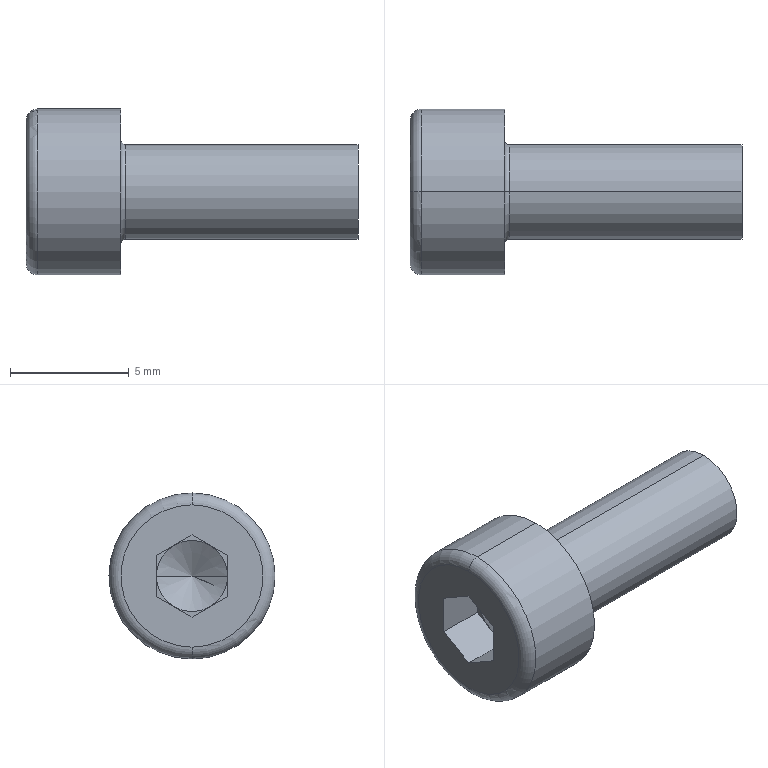Part | NX | features BREP 1 | 1 solid | 25 faces | box 14 x 7 x 7 mm | volume 260.941 mm3 | plane 15 | torus 4 | cylinder 4 | cone 2 | commonest cylinder face diameters 4 x2 7 x2
STEP:
#1=CARTESIAN_POINT('',(0.5,0.,-3.5));
#2=VERTEX_POINT('',#1);
#3=CARTESIAN_POINT('',(0.5,0.,3.5));
#4=VERTEX_POINT('',#3);
#5=CARTESIAN_POINT('',(0.5,0.,0.));
#6=DIRECTION('',(1.,0.,0.));
#7=DIRECTION('',(0.,0.,1.));
#8=AXIS2_PLACEMENT_3D('',#5,#6,#7);
#9=CIRCLE('',#8,3.5);
#10=EDGE_CURVE('',#2,#4,#9,.T.);
#11=ORIENTED_EDGE('',*,*,#10,.F.);
#12=CARTESIAN_POINT('',(0.,0.,-3.));
#13=VERTEX_POINT('',#12);
#14=CARTESIAN_POINT('',(0.5,0.,-3.));
#15=DIRECTION('',(0.,1.,0.));
#16=DIRECTION('',(0.,0.,1.));
#17=AXIS2_PLACEMENT_3D('',#14,#15,#16);
#18=CIRCLE('',#17,0.5);
#19=EDGE_CURVE('',#2,#13,#18,.T.);
#20=ORIENTED_EDGE('',*,*,#19,.T.);
#21=CARTESIAN_POINT('',(0.,0.,3.));
#22=VERTEX_POINT('',#21);
#23=CARTESIAN_POINT('',(0.,0.,0.));
#24=DIRECTION('',(-1.,0.,0.));
#25=DIRECTION('',(0.,0.,1.));
#26=AXIS2_PLACEMENT_3D('',#23,#24,#25);
#27=CIRCLE('',#26,3.);
#28=EDGE_CURVE('',#22,#13,#27,.T.);
#29=ORIENTED_EDGE('',*,*,#28,.F.);
#30=CARTESIAN_POINT('',(0.5,0.,3.));
#31=DIRECTION('',(0.,-1.,0.));
#32=DIRECTION('',(0.,0.,-1.));
#33=AXIS2_PLACEMENT_3D('',#30,#31,#32);
#34=CIRCLE('',#33,0.5);
#35=EDGE_CURVE('',#4,#22,#34,.T.);
#36=ORIENTED_EDGE('',*,*,#35,.F.);
#37=EDGE_LOOP('',(#11,#20,#29,#36));
#38=FACE_BOUND('',#37,.T.);
#39=CARTESIAN_POINT('',(0.5,0.,0.));
#40=DIRECTION('',(-1.,0.,0.));
#41=DIRECTION('',(0.,0.,-1.));
#42=AXIS2_PLACEMENT_3D('',#39,#40,#41);
#43=TOROIDAL_SURFACE('',#42,3.,0.5);
#44=ADVANCED_FACE('',(#38),#43,.T.);
#45=CARTESIAN_POINT('',(4.2,0.,2.));
#46=VERTEX_POINT('',#45);
#47=CARTESIAN_POINT('',(4.2,0.,-2.));
#48=VERTEX_POINT('',#47);
#49=CARTESIAN_POINT('',(4.2,0.,0.));
#50=DIRECTION('',(1.,0.,0.));
#51=DIRECTION('',(0.,0.,-1.));
#52=AXIS2_PLACEMENT_3D('',#49,#50,#51);
#53=CIRCLE('',#52,2.);
#54=EDGE_CURVE('',#46,#48,#53,.T.);
#55=ORIENTED_EDGE('',*,*,#54,.F.);
#56=CARTESIAN_POINT('',(4.,0.,2.2));
#57=VERTEX_POINT('',#56);
#58=CARTESIAN_POINT('',(4.2,0.,2.2));
#59=DIRECTION('',(0.,1.,0.));
#60=DIRECTION('',(0.,0.,1.));
#61=AXIS2_PLACEMENT_3D('',#58,#59,#60);
#62=CIRCLE('',#61,0.2);
#63=EDGE_CURVE('',#57,#46,#62,.F.);
#64=ORIENTED_EDGE('',*,*,#63,.F.);
#65=CARTESIAN_POINT('',(4.,0.,-2.2));
#66=VERTEX_POINT('',#65);
#67=CARTESIAN_POINT('',(4.,0.,0.));
#68=DIRECTION('',(-1.,0.,0.));
#69=DIRECTION('',(0.,0.,-1.));
#70=AXIS2_PLACEMENT_3D('',#67,#68,#69);
#71=CIRCLE('',#70,2.2);
#72=EDGE_CURVE('',#66,#57,#71,.T.);
#73=ORIENTED_EDGE('',*,*,#72,.F.);
#74=CARTESIAN_POINT('',(4.2,0.,-2.2));
#75=DIRECTION('',(0.,-1.,0.));
#76=DIRECTION('',(0.,0.,-1.));
#77=AXIS2_PLACEMENT_3D('',#74,#75,#76);
#78=CIRCLE('',#77,0.2);
#79=EDGE_CURVE('',#66,#48,#78,.F.);
#80=ORIENTED_EDGE('',*,*,#79,.T.);
#81=EDGE_LOOP('',(#55,#64,#73,#80));
#82=FACE_BOUND('',#81,.T.);
#83=CARTESIAN_POINT('',(4.2,0.,0.));
#84=DIRECTION('',(1.,0.,0.));
#85=DIRECTION('',(0.,0.,1.));
#86=AXIS2_PLACEMENT_3D('',#83,#84,#85);
#87=TOROIDAL_SURFACE('',#86,2.2,0.2);
#88=ADVANCED_FACE('',(#82),#87,.F.);
#89=CARTESIAN_POINT('',(2.,-1.5,0.));
#90=VERTEX_POINT('',#89);
#91=CARTESIAN_POINT('',(2.866,0.,0.));
#92=VERTEX_POINT('',#91);
#93=CARTESIAN_POINT('',(2.866,0.,0.));
#94=DIRECTION('',(-0.5,-0.866,0.));
#95=VECTOR('',#94,1000.);
#96=LINE('',#93,#95);
#97=EDGE_CURVE('',#90,#92,#96,.F.);
#98=ORIENTED_EDGE('',*,*,#97,.T.);
#99=CARTESIAN_POINT('',(2.,1.5,0.));
#100=VERTEX_POINT('',#99);
#101=CARTESIAN_POINT('',(2.866,0.,0.));
#102=DIRECTION('',(-0.5,0.866,0.));
#103=VECTOR('',#102,1000.);
#104=LINE('',#101,#103);
#105=EDGE_CURVE('',#100,#92,#104,.F.);
#106=ORIENTED_EDGE('',*,*,#105,.F.);
#107=CARTESIAN_POINT('',(2.,0.75,-1.299));
#108=VERTEX_POINT('',#107);
#109=CARTESIAN_POINT('',(2.,0.,0.));
#110=DIRECTION('',(1.,0.,0.));
#111=DIRECTION('',(0.,1.,0.));
#112=AXIS2_PLACEMENT_3D('',#109,#110,#111);
#113=CIRCLE('',#112,1.5);
#114=EDGE_CURVE('',#108,#100,#113,.T.);
#115=ORIENTED_EDGE('',*,*,#114,.F.);
#116=CARTESIAN_POINT('',(2.,-0.75,-1.299));
#117=VERTEX_POINT('',#116);
#118=CARTESIAN_POINT('',(2.,0.,0.));
#119=DIRECTION('',(1.,0.,0.));
#120=DIRECTION('',(0.,1.,0.));
#121=AXIS2_PLACEMENT_3D('',#118,#119,#120);
#122=CIRCLE('',#121,1.5);
#123=EDGE_CURVE('',#117,#108,#122,.T.);
#124=ORIENTED_EDGE('',*,*,#123,.F.);
#125=CARTESIAN_POINT('',(2.,0.,0.));
#126=DIRECTION('',(1.,0.,0.));
#127=DIRECTION('',(0.,1.,0.));
#128=AXIS2_PLACEMENT_3D('',#125,#126,#127);
#129=CIRCLE('',#128,1.5);
#130=EDGE_CURVE('',#90,#117,#129,.T.);
#131=ORIENTED_EDGE('',*,*,#130,.F.);
#132=EDGE_LOOP('',(#98,#106,#115,#124,#131));
#133=FACE_BOUND('',#132,.T.);
#134=CARTESIAN_POINT('',(-997.134,0.,0.));
#135=DIRECTION('',(-1.,0.,0.));
#136=DIRECTION('',(0.,1.,0.));
#137=AXIS2_PLACEMENT_3D('',#134,#135,#136);
#138=CONICAL_SURFACE('',#137,1732.051,1.047);
#139=ADVANCED_FACE('',(#133),#138,.F.);
#140=CARTESIAN_POINT('',(14.,0.,-2.));
#141=VERTEX_POINT('',#140);
#142=CARTESIAN_POINT('',(14.,0.,2.));
#143=VERTEX_POINT('',#142);
#144=CARTESIAN_POINT('',(14.,0.,0.));
#145=DIRECTION('',(1.,0.,0.));
#146=DIRECTION('',(0.,0.,-1.));
#147=AXIS2_PLACEMENT_3D('',#144,#145,#146);
#148=CIRCLE('',#147,2.);
#149=EDGE_CURVE('',#141,#143,#148,.T.);
#150=ORIENTED_EDGE('',*,*,#149,.F.);
#151=CARTESIAN_POINT('',(10.,0.,-2.));
#152=DIRECTION('',(-1.,0.,0.));
#153=VECTOR('',#152,1000.);
#154=LINE('',#151,#153);
#155=EDGE_CURVE('',#141,#48,#154,.T.);
#156=ORIENTED_EDGE('',*,*,#155,.T.);
#157=CARTESIAN_POINT('',(4.2,0.,0.));
#158=DIRECTION('',(1.,0.,0.));
#159=DIRECTION('',(0.,0.,-1.));
#160=AXIS2_PLACEMENT_3D('',#157,#158,#159);
#161=CIRCLE('',#160,2.);
#162=EDGE_CURVE('',#48,#46,#161,.T.);
#163=ORIENTED_EDGE('',*,*,#162,.T.);
#164=CARTESIAN_POINT('',(10.,0.,2.));
#165=DIRECTION('',(-1.,0.,0.));
#166=VECTOR('',#165,1000.);
#167=LINE('',#164,#166);
#168=EDGE_CURVE('',#143,#46,#167,.T.);
#169=ORIENTED_EDGE('',*,*,#168,.F.);
#170=EDGE_LOOP('',(#150,#156,#163,#169));
#171=FACE_BOUND('',#170,.T.);
#172=CARTESIAN_POINT('',(10.,0.,0.));
#173=DIRECTION('',(-1.,0.,0.));
#174=DIRECTION('',(0.,0.,-1.));
#175=AXIS2_PLACEMENT_3D('',#172,#173,#174);
#176=CYLINDRICAL_SURFACE('',#175,2.);
#177=ADVANCED_FACE('',(#171),#176,.T.);
#178=CARTESIAN_POINT('',(4.,0.,3.5));
#179=VERTEX_POINT('',#178);
#180=CARTESIAN_POINT('',(4.,0.,-3.5));
#181=VERTEX_POINT('',#180);
#182=CARTESIAN_POINT('',(4.,0.,0.));
#183=DIRECTION('',(-1.,0.,0.));
#184=DIRECTION('',(0.,0.,1.));
#185=AXIS2_PLACEMENT_3D('',#182,#183,#184);
#186=CIRCLE('',#185,3.5);
#187=EDGE_CURVE('',#179,#181,#186,.T.);
#188=ORIENTED_EDGE('',*,*,#187,.T.);
#189=CARTESIAN_POINT('',(4.,0.,-3.5));
#190=DIRECTION('',(-1.,0.,0.));
#191=VECTOR('',#190,1000.);
#192=LINE('',#189,#191);
#193=EDGE_CURVE('',#181,#2,#192,.T.);
#194=ORIENTED_EDGE('',*,*,#193,.T.);
#195=ORIENTED_EDGE('',*,*,#10,.T.);
#196=CARTESIAN_POINT('',(4.,0.,3.5));
#197=DIRECTION('',(-1.,0.,0.));
#198=VECTOR('',#197,1000.);
#199=LINE('',#196,#198);
#200=EDGE_CURVE('',#179,#4,#199,.T.);
#201=ORIENTED_EDGE('',*,*,#200,.F.);
#202=EDGE_LOOP('',(#188,#194,#195,#201));
#203=FACE_BOUND('',#202,.T.);
#204=CARTESIAN_POINT('',(4.,0.,0.));
#205=DIRECTION('',(-1.,0.,0.));
#206=DIRECTION('',(0.,0.,-1.));
#207=AXIS2_PLACEMENT_3D('',#204,#205,#206);
#208=CYLINDRICAL_SURFACE('',#207,3.5);
#209=ADVANCED_FACE('',(#203),#208,.T.);
#210=CARTESIAN_POINT('',(2.,1.5,0.866));
#211=VERTEX_POINT('',#210);
#212=CARTESIAN_POINT('',(2.,1.5,0.866));
#213=DIRECTION('',(0.,0.,-1.));
#214=VECTOR('',#213,1000.);
#215=LINE('',#212,#214);
#216=EDGE_CURVE('',#211,#100,#215,.T.);
#217=ORIENTED_EDGE('',*,*,#216,.T.);
#218=CARTESIAN_POINT('',(2.,0.75,1.299));
#219=VERTEX_POINT('',#218);
#220=CARTESIAN_POINT('',(2.,0.,0.));
#221=DIRECTION('',(1.,0.,0.));
#222=DIRECTION('',(0.,1.,0.));
#223=AXIS2_PLACEMENT_3D('',#220,#221,#222);
#224=CIRCLE('',#223,1.5);
#225=EDGE_CURVE('',#100,#219,#224,.T.);
#226=ORIENTED_EDGE('',*,*,#225,.T.);
#227=CARTESIAN_POINT('',(2.,0.,1.732));
#228=DIRECTION('',(0.,0.866,-0.5));
#229=VECTOR('',#228,1000.);
#230=LINE('',#227,#229);
#231=EDGE_CURVE('',#219,#211,#230,.T.);
#232=ORIENTED_EDGE('',*,*,#231,.T.);
#233=EDGE_LOOP('',(#217,#226,#232));
#234=FACE_BOUND('',#233,.T.);
#235=CARTESIAN_POINT('',(2.,0.,0.));
#236=DIRECTION('',(-1.,0.,0.));
#237=DIRECTION('',(0.,0.,-1.));
#238=AXIS2_PLACEMENT_3D('',#235,#236,#237);
#239=PLANE('',#238);
#240=ADVANCED_FACE('',(#234),#239,.T.);
#241=CARTESIAN_POINT('',(2.,0.,1.732));
#242=VERTEX_POINT('',#241);
#243=CARTESIAN_POINT('',(2.,0.,1.732));
#244=DIRECTION('',(0.,0.866,-0.5));
#245=VECTOR('',#244,1000.);
#246=LINE('',#243,#245);
#247=EDGE_CURVE('',#242,#219,#246,.T.);
#248=ORIENTED_EDGE('',*,*,#247,.T.);
#249=CARTESIAN_POINT('',(2.,-0.75,1.299));
#250=VERTEX_POINT('',#249);
#251=CARTESIAN_POINT('',(2.,0.,0.));
#252=DIRECTION('',(1.,0.,0.));
#253=DIRECTION('',(0.,1.,0.));
#254=AXIS2_PLACEMENT_3D('',#251,#252,#253);
#255=CIRCLE('',#254,1.5);
#256=EDGE_CURVE('',#219,#250,#255,.T.);
#257=ORIENTED_EDGE('',*,*,#256,.T.);
#258=CARTESIAN_POINT('',(2.,-1.5,0.866));
#259=DIRECTION('',(0.,0.866,0.5));
#260=VECTOR('',#259,1000.);
#261=LINE('',#258,#260);
#262=EDGE_CURVE('',#250,#242,#261,.T.);
#263=ORIENTED_EDGE('',*,*,#262,.T.);
#264=EDGE_LOOP('',(#248,#257,#263));
#265=FACE_BOUND('',#264,.T.);
#266=CARTESIAN_POINT('',(2.,0.,0.));
#267=DIRECTION('',(-1.,0.,0.));
#268=DIRECTION('',(0.,0.,-1.));
#269=AXIS2_PLACEMENT_3D('',#266,#267,#268);
#270=PLANE('',#269);
#271=ADVANCED_FACE('',(#265),#270,.T.);
#272=CARTESIAN_POINT('',(2.,-1.5,0.866));
#273=VERTEX_POINT('',#272);
#274=CARTESIAN_POINT('',(2.,-1.5,0.866));
#275=DIRECTION('',(0.,0.866,0.5));
#276=VECTOR('',#275,1000.);
#277=LINE('',#274,#276);
#278=EDGE_CURVE('',#273,#250,#277,.T.);
#279=ORIENTED_EDGE('',*,*,#278,.T.);
#280=CARTESIAN_POINT('',(2.,0.,0.));
#281=DIRECTION('',(1.,0.,0.));
#282=DIRECTION('',(0.,1.,0.));
#283=AXIS2_PLACEMENT_3D('',#280,#281,#282);
#284=CIRCLE('',#283,1.5);
#285=EDGE_CURVE('',#250,#90,#284,.T.);
#286=ORIENTED_EDGE('',*,*,#285,.T.);
#287=CARTESIAN_POINT('',(2.,-1.5,-0.866));
#288=DIRECTION('',(0.,0.,1.));
#289=VECTOR('',#288,1000.);
#290=LINE('',#287,#289);
#291=EDGE_CURVE('',#90,#273,#290,.T.);
#292=ORIENTED_EDGE('',*,*,#291,.T.);
#293=EDGE_LOOP('',(#279,#286,#292));
#294=FACE_BOUND('',#293,.T.);
#295=CARTESIAN_POINT('',(2.,0.,0.));
#296=DIRECTION('',(-1.,0.,0.));
#297=DIRECTION('',(0.,0.,-1.));
#298=AXIS2_PLACEMENT_3D('',#295,#296,#297);
#299=PLANE('',#298);
#300=ADVANCED_FACE('',(#294),#299,.T.);
#301=CARTESIAN_POINT('',(2.,-1.5,-0.866));
#302=VERTEX_POINT('',#301);
#303=CARTESIAN_POINT('',(2.,-1.5,-0.866));
#304=DIRECTION('',(0.,0.,1.));
#305=VECTOR('',#304,1000.);
#306=LINE('',#303,#305);
#307=EDGE_CURVE('',#302,#90,#306,.T.);
#308=ORIENTED_EDGE('',*,*,#307,.T.);
#309=ORIENTED_EDGE('',*,*,#130,.T.);
#310=CARTESIAN_POINT('',(2.,0.,-1.732));
#311=DIRECTION('',(0.,-0.866,0.5));
#312=VECTOR('',#311,1000.);
#313=LINE('',#310,#312);
#314=EDGE_CURVE('',#117,#302,#313,.T.);
#315=ORIENTED_EDGE('',*,*,#314,.T.);
#316=EDGE_LOOP('',(#308,#309,#315));
#317=FACE_BOUND('',#316,.T.);
#318=CARTESIAN_POINT('',(2.,0.,0.));
#319=DIRECTION('',(-1.,0.,0.));
#320=DIRECTION('',(0.,0.,-1.));
#321=AXIS2_PLACEMENT_3D('',#318,#319,#320);
#322=PLANE('',#321);
#323=ADVANCED_FACE('',(#317),#322,.T.);
#324=CARTESIAN_POINT('',(2.,0.,-1.732));
#325=VERTEX_POINT('',#324);
#326=CARTESIAN_POINT('',(2.,0.,-1.732));
#327=DIRECTION('',(0.,-0.866,0.5));
#328=VECTOR('',#327,1000.);
#329=LINE('',#326,#328);
#330=EDGE_CURVE('',#325,#117,#329,.T.);
#331=ORIENTED_EDGE('',*,*,#330,.T.);
#332=ORIENTED_EDGE('',*,*,#123,.T.);
#333=CARTESIAN_POINT('',(2.,1.5,-0.866));
#334=DIRECTION('',(0.,-0.866,-0.5));
#335=VECTOR('',#334,1000.);
#336=LINE('',#333,#335);
#337=EDGE_CURVE('',#108,#325,#336,.T.);
#338=ORIENTED_EDGE('',*,*,#337,.T.);
#339=EDGE_LOOP('',(#331,#332,#338));
#340=FACE_BOUND('',#339,.T.);
#341=CARTESIAN_POINT('',(2.,0.,0.));
#342=DIRECTION('',(-1.,0.,0.));
#343=DIRECTION('',(0.,0.,-1.));
#344=AXIS2_PLACEMENT_3D('',#341,#342,#343);
#345=PLANE('',#344);
#346=ADVANCED_FACE('',(#340),#345,.T.);
#347=ORIENTED_EDGE('',*,*,#193,.F.);
#348=CARTESIAN_POINT('',(4.,0.,0.));
#349=DIRECTION('',(-1.,0.,0.));
#350=DIRECTION('',(0.,0.,1.));
#351=AXIS2_PLACEMENT_3D('',#348,#349,#350);
#352=CIRCLE('',#351,3.5);
#353=EDGE_CURVE('',#181,#179,#352,.T.);
#354=ORIENTED_EDGE('',*,*,#353,.T.);
#355=ORIENTED_EDGE('',*,*,#200,.T.);
#356=CARTESIAN_POINT('',(0.5,0.,0.));
#357=DIRECTION('',(1.,0.,0.));
#358=DIRECTION('',(0.,0.,1.));
#359=AXIS2_PLACEMENT_3D('',#356,#357,#358);
#360=CIRCLE('',#359,3.5);
#361=EDGE_CURVE('',#4,#2,#360,.T.);
#362=ORIENTED_EDGE('',*,*,#361,.T.);
#363=EDGE_LOOP('',(#347,#354,#355,#362));
#364=FACE_BOUND('',#363,.T.);
#365=CARTESIAN_POINT('',(4.,0.,0.));
#366=DIRECTION('',(-1.,0.,0.));
#367=DIRECTION('',(0.,0.,-1.));
#368=AXIS2_PLACEMENT_3D('',#365,#366,#367);
#369=CYLINDRICAL_SURFACE('',#368,3.5);
#370=ADVANCED_FACE('',(#364),#369,.T.);
#371=ORIENTED_EDGE('',*,*,#187,.F.);
#372=ORIENTED_EDGE('',*,*,#353,.F.);
#373=EDGE_LOOP('',(#371,#372));
#374=FACE_BOUND('',#373,.T.);
#375=ORIENTED_EDGE('',*,*,#72,.T.);
#376=CARTESIAN_POINT('',(4.,0.,0.));
#377=DIRECTION('',(-1.,0.,0.));
#378=DIRECTION('',(0.,0.,-1.));
#379=AXIS2_PLACEMENT_3D('',#376,#377,#378);
#380=CIRCLE('',#379,2.2);
#381=EDGE_CURVE('',#57,#66,#380,.T.);
#382=ORIENTED_EDGE('',*,*,#381,.T.);
#383=EDGE_LOOP('',(#375,#382));
#384=FACE_BOUND('',#383,.T.);
#385=CARTESIAN_POINT('',(4.,3.5,0.));
#386=DIRECTION('',(1.,0.,0.));
#387=DIRECTION('',(0.,-1.,0.));
#388=AXIS2_PLACEMENT_3D('',#385,#386,#387);
#389=PLANE('',#388);
#390=ADVANCED_FACE('',(#374,#384),#389,.T.);
#391=ORIENTED_EDGE('',*,*,#28,.T.);
#392=CARTESIAN_POINT('',(0.,0.,0.));
#393=DIRECTION('',(-1.,0.,0.));
#394=DIRECTION('',(0.,0.,1.));
#395=AXIS2_PLACEMENT_3D('',#392,#393,#394);
#396=CIRCLE('',#395,3.);
#397=EDGE_CURVE('',#13,#22,#396,.T.);
#398=ORIENTED_EDGE('',*,*,#397,.T.);
#399=EDGE_LOOP('',(#391,#398));
#400=FACE_BOUND('',#399,.T.);
#401=CARTESIAN_POINT('',(0.,0.,1.732));
#402=VERTEX_POINT('',#401);
#403=CARTESIAN_POINT('',(0.,1.5,0.866));
#404=VERTEX_POINT('',#403);
#405=CARTESIAN_POINT('',(0.,0.,1.732));
#406=DIRECTION('',(0.,0.866,-0.5));
#407=VECTOR('',#406,1000.);
#408=LINE('',#405,#407);
#409=EDGE_CURVE('',#402,#404,#408,.T.);
#410=ORIENTED_EDGE('',*,*,#409,.F.);
#411=CARTESIAN_POINT('',(0.,-1.5,0.866));
#412=VERTEX_POINT('',#411);
#413=CARTESIAN_POINT('',(0.,-1.5,0.866));
#414=DIRECTION('',(0.,0.866,0.5));
#415=VECTOR('',#414,1000.);
#416=LINE('',#413,#415);
#417=EDGE_CURVE('',#412,#402,#416,.T.);
#418=ORIENTED_EDGE('',*,*,#417,.F.);
#419=CARTESIAN_POINT('',(0.,-1.5,-0.866));
#420=VERTEX_POINT('',#419);
#421=CARTESIAN_POINT('',(0.,-1.5,-0.866));
#422=DIRECTION('',(0.,0.,1.));
#423=VECTOR('',#422,1000.);
#424=LINE('',#421,#423);
#425=EDGE_CURVE('',#420,#412,#424,.T.);
#426=ORIENTED_EDGE('',*,*,#425,.F.);
#427=CARTESIAN_POINT('',(0.,0.,-1.732));
#428=VERTEX_POINT('',#427);
#429=CARTESIAN_POINT('',(0.,0.,-1.732));
#430=DIRECTION('',(0.,-0.866,0.5));
#431=VECTOR('',#430,1000.);
#432=LINE('',#429,#431);
#433=EDGE_CURVE('',#428,#420,#432,.T.);
#434=ORIENTED_EDGE('',*,*,#433,.F.);
#435=CARTESIAN_POINT('',(0.,1.5,-0.866));
#436=VERTEX_POINT('',#435);
#437=CARTESIAN_POINT('',(0.,1.5,-0.866));
#438=DIRECTION('',(0.,-0.866,-0.5));
#439=VECTOR('',#438,1000.);
#440=LINE('',#437,#439);
#441=EDGE_CURVE('',#436,#428,#440,.T.);
#442=ORIENTED_EDGE('',*,*,#441,.F.);
#443=CARTESIAN_POINT('',(0.,1.5,0.866));
#444=DIRECTION('',(0.,0.,-1.));
#445=VECTOR('',#444,1000.);
#446=LINE('',#443,#445);
#447=EDGE_CURVE('',#404,#436,#446,.T.);
#448=ORIENTED_EDGE('',*,*,#447,.F.);
#449=EDGE_LOOP('',(#410,#418,#426,#434,#442,#448));
#450=FACE_BOUND('',#449,.T.);
#451=CARTESIAN_POINT('',(0.,0.,0.));
#452=DIRECTION('',(-1.,0.,0.));
#453=DIRECTION('',(0.,0.,-1.));
#454=AXIS2_PLACEMENT_3D('',#451,#452,#453);
#455=PLANE('',#454);
#456=ADVANCED_FACE('',(#400,#450),#455,.T.);
#457=ORIENTED_EDGE('',*,*,#155,.F.);
#458=CARTESIAN_POINT('',(14.,0.,0.));
#459=DIRECTION('',(1.,0.,0.));
#460=DIRECTION('',(0.,0.,-1.));
#461=AXIS2_PLACEMENT_3D('',#458,#459,#460);
#462=CIRCLE('',#461,2.);
#463=EDGE_CURVE('',#143,#141,#462,.T.);
#464=ORIENTED_EDGE('',*,*,#463,.F.);
#465=ORIENTED_EDGE('',*,*,#168,.T.);
#466=ORIENTED_EDGE('',*,*,#54,.T.);
#467=EDGE_LOOP('',(#457,#464,#465,#466));
#468=FACE_BOUND('',#467,.T.);
#469=CARTESIAN_POINT('',(10.,0.,0.));
#470=DIRECTION('',(-1.,0.,0.));
#471=DIRECTION('',(0.,0.,-1.));
#472=AXIS2_PLACEMENT_3D('',#469,#470,#471);
#473=CYLINDRICAL_SURFACE('',#472,2.);
#474=ADVANCED_FACE('',(#468),#473,.T.);
#475=ORIENTED_EDGE('',*,*,#409,.T.);
#476=CARTESIAN_POINT('',(2.,1.5,0.866));
#477=DIRECTION('',(-1.,0.,0.));
#478=VECTOR('',#477,1000.);
#479=LINE('',#476,#478);
#480=EDGE_CURVE('',#211,#404,#479,.T.);
#481=ORIENTED_EDGE('',*,*,#480,.F.);
#482=ORIENTED_EDGE('',*,*,#231,.F.);
#483=ORIENTED_EDGE('',*,*,#247,.F.);
#484=CARTESIAN_POINT('',(2.,0.,1.732));
#485=DIRECTION('',(-1.,0.,0.));
#486=VECTOR('',#485,1000.);
#487=LINE('',#484,#486);
#488=EDGE_CURVE('',#242,#402,#487,.T.);
#489=ORIENTED_EDGE('',*,*,#488,.T.);
#490=EDGE_LOOP('',(#475,#481,#482,#483,#489));
#491=FACE_BOUND('',#490,.T.);
#492=CARTESIAN_POINT('',(2.,0.,1.732));
#493=DIRECTION('',(0.,0.5,0.866));
#494=DIRECTION('',(-1.,0.,0.));
#495=AXIS2_PLACEMENT_3D('',#492,#493,#494);
#496=PLANE('',#495);
#497=ADVANCED_FACE('',(#491),#496,.F.);
#498=ORIENTED_EDGE('',*,*,#417,.T.);
#499=ORIENTED_EDGE('',*,*,#488,.F.);
#500=ORIENTED_EDGE('',*,*,#262,.F.);
#501=ORIENTED_EDGE('',*,*,#278,.F.);
#502=CARTESIAN_POINT('',(2.,-1.5,0.866));
#503=DIRECTION('',(-1.,0.,0.));
#504=VECTOR('',#503,1000.);
#505=LINE('',#502,#504);
#506=EDGE_CURVE('',#273,#412,#505,.T.);
#507=ORIENTED_EDGE('',*,*,#506,.T.);
#508=EDGE_LOOP('',(#498,#499,#500,#501,#507));
#509=FACE_BOUND('',#508,.T.);
#510=CARTESIAN_POINT('',(2.,-1.5,0.866));
#511=DIRECTION('',(0.,-0.5,0.866));
#512=DIRECTION('',(1.,0.,0.));
#513=AXIS2_PLACEMENT_3D('',#510,#511,#512);
#514=PLANE('',#513);
#515=ADVANCED_FACE('',(#509),#514,.F.);
#516=ORIENTED_EDGE('',*,*,#425,.T.);
#517=ORIENTED_EDGE('',*,*,#506,.F.);
#518=ORIENTED_EDGE('',*,*,#291,.F.);
#519=ORIENTED_EDGE('',*,*,#307,.F.);
#520=CARTESIAN_POINT('',(2.,-1.5,-0.866));
#521=DIRECTION('',(-1.,0.,0.));
#522=VECTOR('',#521,1000.);
#523=LINE('',#520,#522);
#524=EDGE_CURVE('',#302,#420,#523,.T.);
#525=ORIENTED_EDGE('',*,*,#524,.T.);
#526=EDGE_LOOP('',(#516,#517,#518,#519,#525));
#527=FACE_BOUND('',#526,.T.);
#528=CARTESIAN_POINT('',(2.,-1.5,-0.866));
#529=DIRECTION('',(0.,-1.,0.));
#530=DIRECTION('',(0.,0.,1.));
#531=AXIS2_PLACEMENT_3D('',#528,#529,#530);
#532=PLANE('',#531);
#533=ADVANCED_FACE('',(#527),#532,.F.);
#534=ORIENTED_EDGE('',*,*,#433,.T.);
#535=ORIENTED_EDGE('',*,*,#524,.F.);
#536=ORIENTED_EDGE('',*,*,#314,.F.);
#537=ORIENTED_EDGE('',*,*,#330,.F.);
#538=CARTESIAN_POINT('',(2.,0.,-1.732));
#539=DIRECTION('',(-1.,0.,0.));
#540=VECTOR('',#539,1000.);
#541=LINE('',#538,#540);
#542=EDGE_CURVE('',#325,#428,#541,.T.);
#543=ORIENTED_EDGE('',*,*,#542,.T.);
#544=EDGE_LOOP('',(#534,#535,#536,#537,#543));
#545=FACE_BOUND('',#544,.T.);
#546=CARTESIAN_POINT('',(2.,0.,-1.732));
#547=DIRECTION('',(0.,-0.5,-0.866));
#548=DIRECTION('',(0.,0.866,-0.5));
#549=AXIS2_PLACEMENT_3D('',#546,#547,#548);
#550=PLANE('',#549);
#551=ADVANCED_FACE('',(#545),#550,.F.);
#552=ORIENTED_EDGE('',*,*,#441,.T.);
#553=ORIENTED_EDGE('',*,*,#542,.F.);
#554=ORIENTED_EDGE('',*,*,#337,.F.);
#555=CARTESIAN_POINT('',(2.,1.5,-0.866));
#556=VERTEX_POINT('',#555);
#557=CARTESIAN_POINT('',(2.,1.5,-0.866));
#558=DIRECTION('',(0.,-0.866,-0.5));
#559=VECTOR('',#558,1000.);
#560=LINE('',#557,#559);
#561=EDGE_CURVE('',#556,#108,#560,.T.);
#562=ORIENTED_EDGE('',*,*,#561,.F.);
#563=CARTESIAN_POINT('',(2.,1.5,-0.866));
#564=DIRECTION('',(-1.,0.,0.));
#565=VECTOR('',#564,1000.);
#566=LINE('',#563,#565);
#567=EDGE_CURVE('',#556,#436,#566,.T.);
#568=ORIENTED_EDGE('',*,*,#567,.T.);
#569=EDGE_LOOP('',(#552,#553,#554,#562,#568));
#570=FACE_BOUND('',#569,.T.);
#571=CARTESIAN_POINT('',(2.,1.5,-0.866));
#572=DIRECTION('',(0.,0.5,-0.866));
#573=DIRECTION('',(1.,0.,0.));
#574=AXIS2_PLACEMENT_3D('',#571,#572,#573);
#575=PLANE('',#574);
#576=ADVANCED_FACE('',(#570),#575,.F.);
#577=ORIENTED_EDGE('',*,*,#447,.T.);
#578=ORIENTED_EDGE('',*,*,#567,.F.);
#579=CARTESIAN_POINT('',(2.,1.5,0.866));
#580=DIRECTION('',(0.,0.,-1.));
#581=VECTOR('',#580,1000.);
#582=LINE('',#579,#581);
#583=EDGE_CURVE('',#100,#556,#582,.T.);
#584=ORIENTED_EDGE('',*,*,#583,.F.);
#585=ORIENTED_EDGE('',*,*,#216,.F.);
#586=ORIENTED_EDGE('',*,*,#480,.T.);
#587=EDGE_LOOP('',(#577,#578,#584,#585,#586));
#588=FACE_BOUND('',#587,.T.);
#589=CARTESIAN_POINT('',(2.,1.5,0.866));
#590=DIRECTION('',(0.,1.,0.));
#591=DIRECTION('',(-1.,0.,0.));
#592=AXIS2_PLACEMENT_3D('',#589,#590,#591);
#593=PLANE('',#592);
#594=ADVANCED_FACE('',(#588),#593,.F.);
#595=ORIENTED_EDGE('',*,*,#561,.T.);
#596=ORIENTED_EDGE('',*,*,#114,.T.);
#597=ORIENTED_EDGE('',*,*,#583,.T.);
#598=EDGE_LOOP('',(#595,#596,#597));
#599=FACE_BOUND('',#598,.T.);
#600=CARTESIAN_POINT('',(2.,0.,0.));
#601=DIRECTION('',(-1.,0.,0.));
#602=DIRECTION('',(0.,0.,-1.));
#603=AXIS2_PLACEMENT_3D('',#600,#601,#602);
#604=PLANE('',#603);
#605=ADVANCED_FACE('',(#599),#604,.T.);
#606=ORIENTED_EDGE('',*,*,#105,.T.);
#607=ORIENTED_EDGE('',*,*,#97,.F.);
#608=ORIENTED_EDGE('',*,*,#285,.F.);
#609=ORIENTED_EDGE('',*,*,#256,.F.);
#610=ORIENTED_EDGE('',*,*,#225,.F.);
#611=EDGE_LOOP('',(#606,#607,#608,#609,#610));
#612=FACE_BOUND('',#611,.T.);
#613=CARTESIAN_POINT('',(-997.134,0.,0.));
#614=DIRECTION('',(-1.,0.,0.));
#615=DIRECTION('',(0.,1.,0.));
#616=AXIS2_PLACEMENT_3D('',#613,#614,#615);
#617=CONICAL_SURFACE('',#616,1732.051,1.047);
#618=ADVANCED_FACE('',(#612),#617,.F.);
#619=ORIENTED_EDGE('',*,*,#63,.T.);
#620=ORIENTED_EDGE('',*,*,#162,.F.);
#621=ORIENTED_EDGE('',*,*,#79,.F.);
#622=ORIENTED_EDGE('',*,*,#381,.F.);
#623=EDGE_LOOP('',(#619,#620,#621,#622));
#624=FACE_BOUND('',#623,.T.);
#625=CARTESIAN_POINT('',(4.2,0.,0.));
#626=DIRECTION('',(1.,0.,0.));
#627=DIRECTION('',(0.,0.,1.));
#628=AXIS2_PLACEMENT_3D('',#625,#626,#627);
#629=TOROIDAL_SURFACE('',#628,2.2,0.2);
#630=ADVANCED_FACE('',(#624),#629,.F.);
#631=ORIENTED_EDGE('',*,*,#19,.F.);
#632=ORIENTED_EDGE('',*,*,#361,.F.);
#633=ORIENTED_EDGE('',*,*,#35,.T.);
#634=ORIENTED_EDGE('',*,*,#397,.F.);
#635=EDGE_LOOP('',(#631,#632,#633,#634));
#636=FACE_BOUND('',#635,.T.);
#637=CARTESIAN_POINT('',(0.5,0.,0.));
#638=DIRECTION('',(-1.,0.,0.));
#639=DIRECTION('',(0.,0.,-1.));
#640=AXIS2_PLACEMENT_3D('',#637,#638,#639);
#641=TOROIDAL_SURFACE('',#640,3.,0.5);
#642=ADVANCED_FACE('',(#636),#641,.T.);
#643=ORIENTED_EDGE('',*,*,#463,.T.);
#644=ORIENTED_EDGE('',*,*,#149,.T.);
#645=EDGE_LOOP('',(#643,#644));
#646=FACE_BOUND('',#645,.T.);
#647=CARTESIAN_POINT('',(14.,0.,0.));
#648=DIRECTION('',(1.,0.,0.));
#649=DIRECTION('',(0.,-1.,0.));
#650=AXIS2_PLACEMENT_3D('',#647,#648,#649);
#651=PLANE('',#650);
#652=ADVANCED_FACE('',(#646),#651,.T.);
#653=CLOSED_SHELL('',(#44,#88,#139,#177,#209,#240,#271,#300,#323,#346,#370,#390,#456,#474,#497,#515,#533,#551,#576,#594,#605,#618,#630,#642,#652));
#654=MANIFOLD_SOLID_BREP('',#653);
#655=(LENGTH_UNIT()NAMED_UNIT(*)SI_UNIT(.MILLI.,.METRE.));
#656=UNCERTAINTY_MEASURE_WITH_UNIT(LENGTH_MEASURE(0.00001),#655,'','');
#657=(NAMED_UNIT(*)PLANE_ANGLE_UNIT()SI_UNIT($,.RADIAN.));
#658=(NAMED_UNIT(*)SI_UNIT($,.STERADIAN.)SOLID_ANGLE_UNIT());
#659=(GEOMETRIC_REPRESENTATION_CONTEXT(3)GLOBAL_UNCERTAINTY_ASSIGNED_CONTEXT((#656))GLOBAL_UNIT_ASSIGNED_CONTEXT((#655,#657,#658))REPRESENTATION_CONTEXT('',''));
#660=ADVANCED_BREP_SHAPE_REPRESENTATION('',(#654),#659);